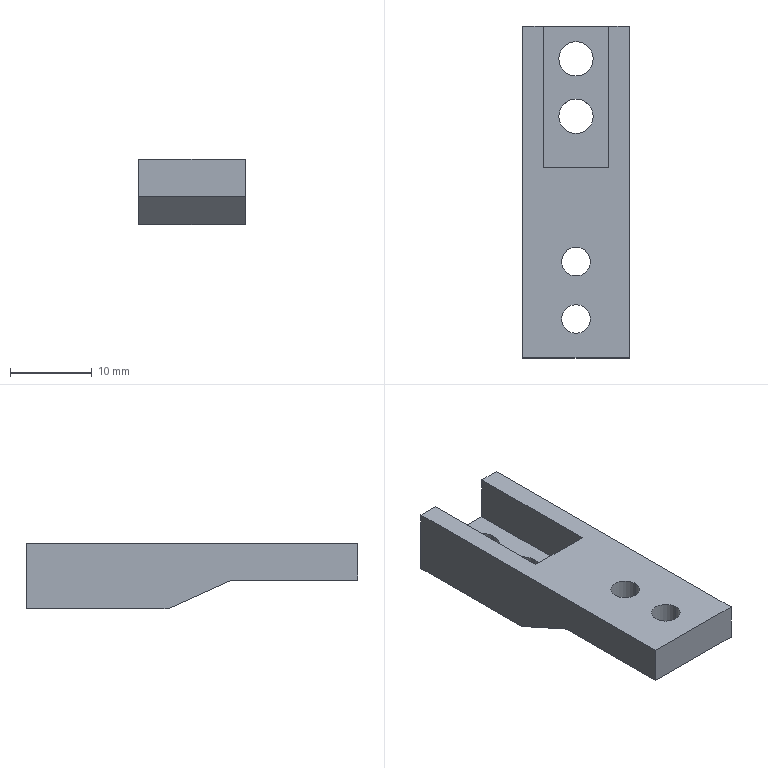Part | 1 solid | 28 faces | box 13 x 40.5 x 8 mm | volume 2407 mm3 | cylinder 12 | plane 12 | cone 4 | commonest cylinder face diameters 3.5 x4 4 x4 4.2 x4
STEP:
#1=CARTESIAN_POINT('',(1.75,-8.5,13.25));
#2=VERTEX_POINT('',#1);
#3=CARTESIAN_POINT('',(-1.75,-8.5,13.25));
#4=VERTEX_POINT('',#3);
#5=CARTESIAN_POINT('',(0.,-8.5,13.25));
#6=DIRECTION('',(0.,0.,-1.));
#7=DIRECTION('',(-1.,0.,0.));
#8=AXIS2_PLACEMENT_3D('',#5,#6,#7);
#9=CIRCLE('',#8,1.75);
#10=EDGE_CURVE('',#2,#4,#9,.T.);
#11=ORIENTED_EDGE('',*,*,#10,.F.);
#12=CARTESIAN_POINT('',(2.,-8.5,13.));
#13=VERTEX_POINT('',#12);
#14=CARTESIAN_POINT('',(2.,-8.5,13.));
#15=DIRECTION('',(0.7071,0.,-0.7071));
#16=VECTOR('',#15,1000.);
#17=LINE('',#14,#16);
#18=EDGE_CURVE('',#2,#13,#17,.T.);
#19=ORIENTED_EDGE('',*,*,#18,.T.);
#20=CARTESIAN_POINT('',(-2.,-8.5,13.));
#21=VERTEX_POINT('',#20);
#22=CARTESIAN_POINT('',(0.,-8.5,13.));
#23=DIRECTION('',(0.,0.,-1.));
#24=DIRECTION('',(-1.,0.,0.));
#25=AXIS2_PLACEMENT_3D('',#22,#23,#24);
#26=CIRCLE('',#25,2.);
#27=EDGE_CURVE('',#13,#21,#26,.T.);
#28=ORIENTED_EDGE('',*,*,#27,.T.);
#29=CARTESIAN_POINT('',(-2.,-8.5,13.));
#30=DIRECTION('',(-0.7071,0.,-0.7071));
#31=VECTOR('',#30,1000.);
#32=LINE('',#29,#31);
#33=EDGE_CURVE('',#4,#21,#32,.T.);
#34=ORIENTED_EDGE('',*,*,#33,.F.);
#35=EDGE_LOOP('',(#11,#19,#28,#34));
#36=FACE_OUTER_BOUND('',#35,.T.);
#37=CARTESIAN_POINT('',(0.,-8.5,13.));
#38=DIRECTION('',(0.,0.,-1.));
#39=DIRECTION('',(-1.,0.,0.));
#40=AXIS2_PLACEMENT_3D('',#37,#38,#39);
#41=CONICAL_SURFACE('',#40,2.,0.7854);
#42=ADVANCED_FACE('',(#36),#41,.F.);
#43=CARTESIAN_POINT('',(1.75,-15.5,13.25));
#44=VERTEX_POINT('',#43);
#45=CARTESIAN_POINT('',(-1.75,-15.5,13.25));
#46=VERTEX_POINT('',#45);
#47=CARTESIAN_POINT('',(0.,-15.5,13.25));
#48=DIRECTION('',(0.,0.,-1.));
#49=DIRECTION('',(-1.,0.,0.));
#50=AXIS2_PLACEMENT_3D('',#47,#48,#49);
#51=CIRCLE('',#50,1.75);
#52=EDGE_CURVE('',#44,#46,#51,.T.);
#53=ORIENTED_EDGE('',*,*,#52,.F.);
#54=CARTESIAN_POINT('',(2.,-15.5,13.));
#55=VERTEX_POINT('',#54);
#56=CARTESIAN_POINT('',(2.,-15.5,13.));
#57=DIRECTION('',(0.7071,0.,-0.7071));
#58=VECTOR('',#57,1000.);
#59=LINE('',#56,#58);
#60=EDGE_CURVE('',#44,#55,#59,.T.);
#61=ORIENTED_EDGE('',*,*,#60,.T.);
#62=CARTESIAN_POINT('',(-2.,-15.5,13.));
#63=VERTEX_POINT('',#62);
#64=CARTESIAN_POINT('',(0.,-15.5,13.));
#65=DIRECTION('',(0.,0.,-1.));
#66=DIRECTION('',(-1.,0.,0.));
#67=AXIS2_PLACEMENT_3D('',#64,#65,#66);
#68=CIRCLE('',#67,2.);
#69=EDGE_CURVE('',#55,#63,#68,.T.);
#70=ORIENTED_EDGE('',*,*,#69,.T.);
#71=CARTESIAN_POINT('',(-2.,-15.5,13.));
#72=DIRECTION('',(-0.7071,0.,-0.7071));
#73=VECTOR('',#72,1000.);
#74=LINE('',#71,#73);
#75=EDGE_CURVE('',#46,#63,#74,.T.);
#76=ORIENTED_EDGE('',*,*,#75,.F.);
#77=EDGE_LOOP('',(#53,#61,#70,#76));
#78=FACE_OUTER_BOUND('',#77,.T.);
#79=CARTESIAN_POINT('',(0.,-15.5,13.));
#80=DIRECTION('',(0.,0.,-1.));
#81=DIRECTION('',(-1.,0.,0.));
#82=AXIS2_PLACEMENT_3D('',#79,#80,#81);
#83=CONICAL_SURFACE('',#82,2.,0.7854);
#84=ADVANCED_FACE('',(#78),#83,.F.);
#85=ORIENTED_EDGE('',*,*,#69,.F.);
#86=CARTESIAN_POINT('',(2.,-15.5,11.5));
#87=VERTEX_POINT('',#86);
#88=CARTESIAN_POINT('',(2.,-15.5,13.));
#89=DIRECTION('',(0.,0.,-1.));
#90=VECTOR('',#89,1000.);
#91=LINE('',#88,#90);
#92=EDGE_CURVE('',#55,#87,#91,.T.);
#93=ORIENTED_EDGE('',*,*,#92,.T.);
#94=CARTESIAN_POINT('',(-2.,-15.5,11.5));
#95=VERTEX_POINT('',#94);
#96=CARTESIAN_POINT('',(0.,-15.5,11.5));
#97=DIRECTION('',(0.,0.,-1.));
#98=DIRECTION('',(-1.,0.,0.));
#99=AXIS2_PLACEMENT_3D('',#96,#97,#98);
#100=CIRCLE('',#99,2.);
#101=EDGE_CURVE('',#87,#95,#100,.T.);
#102=ORIENTED_EDGE('',*,*,#101,.T.);
#103=CARTESIAN_POINT('',(-2.,-15.5,13.));
#104=DIRECTION('',(0.,0.,-1.));
#105=VECTOR('',#104,1000.);
#106=LINE('',#103,#105);
#107=EDGE_CURVE('',#63,#95,#106,.T.);
#108=ORIENTED_EDGE('',*,*,#107,.F.);
#109=EDGE_LOOP('',(#85,#93,#102,#108));
#110=FACE_OUTER_BOUND('',#109,.T.);
#111=CARTESIAN_POINT('',(0.,-15.5,13.));
#112=DIRECTION('',(0.,0.,-1.));
#113=DIRECTION('',(-1.,0.,0.));
#114=AXIS2_PLACEMENT_3D('',#111,#112,#113);
#115=CYLINDRICAL_SURFACE('',#114,2.);
#116=ADVANCED_FACE('',(#110),#115,.F.);
#117=ORIENTED_EDGE('',*,*,#27,.F.);
#118=CARTESIAN_POINT('',(2.,-8.5,11.5));
#119=VERTEX_POINT('',#118);
#120=CARTESIAN_POINT('',(2.,-8.5,13.));
#121=DIRECTION('',(0.,0.,-1.));
#122=VECTOR('',#121,1000.);
#123=LINE('',#120,#122);
#124=EDGE_CURVE('',#13,#119,#123,.T.);
#125=ORIENTED_EDGE('',*,*,#124,.T.);
#126=CARTESIAN_POINT('',(-2.,-8.5,11.5));
#127=VERTEX_POINT('',#126);
#128=CARTESIAN_POINT('',(0.,-8.5,11.5));
#129=DIRECTION('',(0.,0.,-1.));
#130=DIRECTION('',(-1.,0.,0.));
#131=AXIS2_PLACEMENT_3D('',#128,#129,#130);
#132=CIRCLE('',#131,2.);
#133=EDGE_CURVE('',#119,#127,#132,.T.);
#134=ORIENTED_EDGE('',*,*,#133,.T.);
#135=CARTESIAN_POINT('',(-2.,-8.5,13.));
#136=DIRECTION('',(0.,0.,-1.));
#137=VECTOR('',#136,1000.);
#138=LINE('',#135,#137);
#139=EDGE_CURVE('',#21,#127,#138,.T.);
#140=ORIENTED_EDGE('',*,*,#139,.F.);
#141=EDGE_LOOP('',(#117,#125,#134,#140));
#142=FACE_OUTER_BOUND('',#141,.T.);
#143=CARTESIAN_POINT('',(0.,-8.5,13.));
#144=DIRECTION('',(0.,0.,-1.));
#145=DIRECTION('',(-1.,0.,0.));
#146=AXIS2_PLACEMENT_3D('',#143,#144,#145);
#147=CYLINDRICAL_SURFACE('',#146,2.);
#148=ADVANCED_FACE('',(#142),#147,.F.);
#149=CARTESIAN_POINT('',(-2.1,9.25,8.));
#150=VERTEX_POINT('',#149);
#151=CARTESIAN_POINT('',(2.1,9.25,8.));
#152=VERTEX_POINT('',#151);
#153=CARTESIAN_POINT('',(0.,9.25,8.));
#154=DIRECTION('',(0.,0.,1.));
#155=DIRECTION('',(0.,-1.,0.));
#156=AXIS2_PLACEMENT_3D('',#153,#154,#155);
#157=CIRCLE('',#156,2.1);
#158=EDGE_CURVE('',#150,#152,#157,.T.);
#159=ORIENTED_EDGE('',*,*,#158,.F.);
#160=CARTESIAN_POINT('',(-2.1,9.25,10.5));
#161=VERTEX_POINT('',#160);
#162=CARTESIAN_POINT('',(-2.1,9.25,0.5));
#163=DIRECTION('',(0.,0.,1.));
#164=VECTOR('',#163,1000.);
#165=LINE('',#162,#164);
#166=EDGE_CURVE('',#150,#161,#165,.T.);
#167=ORIENTED_EDGE('',*,*,#166,.T.);
#168=CARTESIAN_POINT('',(2.1,9.25,10.5));
#169=VERTEX_POINT('',#168);
#170=CARTESIAN_POINT('',(0.,9.25,10.5));
#171=DIRECTION('',(0.,0.,1.));
#172=DIRECTION('',(1.,0.,0.));
#173=AXIS2_PLACEMENT_3D('',#170,#171,#172);
#174=CIRCLE('',#173,2.1);
#175=EDGE_CURVE('',#161,#169,#174,.T.);
#176=ORIENTED_EDGE('',*,*,#175,.T.);
#177=CARTESIAN_POINT('',(2.1,9.25,0.5));
#178=DIRECTION('',(0.,0.,1.));
#179=VECTOR('',#178,1000.);
#180=LINE('',#177,#179);
#181=EDGE_CURVE('',#152,#169,#180,.T.);
#182=ORIENTED_EDGE('',*,*,#181,.F.);
#183=EDGE_LOOP('',(#159,#167,#176,#182));
#184=FACE_OUTER_BOUND('',#183,.T.);
#185=CARTESIAN_POINT('',(0.,9.25,0.5));
#186=DIRECTION('',(0.,0.,1.));
#187=DIRECTION('',(1.,0.,0.));
#188=AXIS2_PLACEMENT_3D('',#185,#186,#187);
#189=CYLINDRICAL_SURFACE('',#188,2.1);
#190=ADVANCED_FACE('',(#184),#189,.F.);
#191=CARTESIAN_POINT('',(-2.1,16.25,8.));
#192=VERTEX_POINT('',#191);
#193=CARTESIAN_POINT('',(2.1,16.25,8.));
#194=VERTEX_POINT('',#193);
#195=CARTESIAN_POINT('',(0.,16.25,8.));
#196=DIRECTION('',(0.,0.,1.));
#197=DIRECTION('',(0.,-1.,0.));
#198=AXIS2_PLACEMENT_3D('',#195,#196,#197);
#199=CIRCLE('',#198,2.1);
#200=EDGE_CURVE('',#192,#194,#199,.T.);
#201=ORIENTED_EDGE('',*,*,#200,.F.);
#202=CARTESIAN_POINT('',(-2.1,16.25,10.5));
#203=VERTEX_POINT('',#202);
#204=CARTESIAN_POINT('',(-2.1,16.25,0.5));
#205=DIRECTION('',(0.,0.,1.));
#206=VECTOR('',#205,1000.);
#207=LINE('',#204,#206);
#208=EDGE_CURVE('',#192,#203,#207,.T.);
#209=ORIENTED_EDGE('',*,*,#208,.T.);
#210=CARTESIAN_POINT('',(2.1,16.25,10.5));
#211=VERTEX_POINT('',#210);
#212=CARTESIAN_POINT('',(0.,16.25,10.5));
#213=DIRECTION('',(0.,0.,1.));
#214=DIRECTION('',(1.,0.,0.));
#215=AXIS2_PLACEMENT_3D('',#212,#213,#214);
#216=CIRCLE('',#215,2.1);
#217=EDGE_CURVE('',#203,#211,#216,.T.);
#218=ORIENTED_EDGE('',*,*,#217,.T.);
#219=CARTESIAN_POINT('',(2.1,16.25,0.5));
#220=DIRECTION('',(0.,0.,1.));
#221=VECTOR('',#220,1000.);
#222=LINE('',#219,#221);
#223=EDGE_CURVE('',#194,#211,#222,.T.);
#224=ORIENTED_EDGE('',*,*,#223,.F.);
#225=EDGE_LOOP('',(#201,#209,#218,#224));
#226=FACE_OUTER_BOUND('',#225,.T.);
#227=CARTESIAN_POINT('',(0.,16.25,0.5));
#228=DIRECTION('',(0.,0.,1.));
#229=DIRECTION('',(1.,0.,0.));
#230=AXIS2_PLACEMENT_3D('',#227,#228,#229);
#231=CYLINDRICAL_SURFACE('',#230,2.1);
#232=ADVANCED_FACE('',(#226),#231,.F.);
#233=CARTESIAN_POINT('',(1.75,-8.5,16.));
#234=VERTEX_POINT('',#233);
#235=CARTESIAN_POINT('',(-1.75,-8.5,16.));
#236=VERTEX_POINT('',#235);
#237=CARTESIAN_POINT('',(0.,-8.5,16.));
#238=DIRECTION('',(0.,0.,-1.));
#239=DIRECTION('',(-1.,0.,0.));
#240=AXIS2_PLACEMENT_3D('',#237,#238,#239);
#241=CIRCLE('',#240,1.75);
#242=EDGE_CURVE('',#234,#236,#241,.T.);
#243=ORIENTED_EDGE('',*,*,#242,.F.);
#244=CARTESIAN_POINT('',(1.75,-8.5,51.5));
#245=DIRECTION('',(0.,0.,-1.));
#246=VECTOR('',#245,1000.);
#247=LINE('',#244,#246);
#248=EDGE_CURVE('',#234,#2,#247,.T.);
#249=ORIENTED_EDGE('',*,*,#248,.T.);
#250=ORIENTED_EDGE('',*,*,#10,.T.);
#251=CARTESIAN_POINT('',(-1.75,-8.5,51.5));
#252=DIRECTION('',(0.,0.,-1.));
#253=VECTOR('',#252,1000.);
#254=LINE('',#251,#253);
#255=EDGE_CURVE('',#236,#4,#254,.T.);
#256=ORIENTED_EDGE('',*,*,#255,.F.);
#257=EDGE_LOOP('',(#243,#249,#250,#256));
#258=FACE_OUTER_BOUND('',#257,.T.);
#259=CARTESIAN_POINT('',(0.,-8.5,51.5));
#260=DIRECTION('',(0.,0.,-1.));
#261=DIRECTION('',(-1.,0.,0.));
#262=AXIS2_PLACEMENT_3D('',#259,#260,#261);
#263=CYLINDRICAL_SURFACE('',#262,1.75);
#264=ADVANCED_FACE('',(#258),#263,.F.);
#265=CARTESIAN_POINT('',(1.75,-15.5,16.));
#266=VERTEX_POINT('',#265);
#267=CARTESIAN_POINT('',(-1.75,-15.5,16.));
#268=VERTEX_POINT('',#267);
#269=CARTESIAN_POINT('',(0.,-15.5,16.));
#270=DIRECTION('',(0.,0.,-1.));
#271=DIRECTION('',(-1.,0.,0.));
#272=AXIS2_PLACEMENT_3D('',#269,#270,#271);
#273=CIRCLE('',#272,1.75);
#274=EDGE_CURVE('',#266,#268,#273,.T.);
#275=ORIENTED_EDGE('',*,*,#274,.F.);
#276=CARTESIAN_POINT('',(1.75,-15.5,51.5));
#277=DIRECTION('',(0.,0.,-1.));
#278=VECTOR('',#277,1000.);
#279=LINE('',#276,#278);
#280=EDGE_CURVE('',#266,#44,#279,.T.);
#281=ORIENTED_EDGE('',*,*,#280,.T.);
#282=ORIENTED_EDGE('',*,*,#52,.T.);
#283=CARTESIAN_POINT('',(-1.75,-15.5,51.5));
#284=DIRECTION('',(0.,0.,-1.));
#285=VECTOR('',#284,1000.);
#286=LINE('',#283,#285);
#287=EDGE_CURVE('',#268,#46,#286,.T.);
#288=ORIENTED_EDGE('',*,*,#287,.F.);
#289=EDGE_LOOP('',(#275,#281,#282,#288));
#290=FACE_OUTER_BOUND('',#289,.T.);
#291=CARTESIAN_POINT('',(0.,-15.5,51.5));
#292=DIRECTION('',(0.,0.,-1.));
#293=DIRECTION('',(-1.,0.,0.));
#294=AXIS2_PLACEMENT_3D('',#291,#292,#293);
#295=CYLINDRICAL_SURFACE('',#294,1.75);
#296=ADVANCED_FACE('',(#290),#295,.F.);
#297=ORIENTED_EDGE('',*,*,#280,.F.);
#298=CARTESIAN_POINT('',(0.,-15.5,16.));
#299=DIRECTION('',(0.,0.,-1.));
#300=DIRECTION('',(-1.,0.,0.));
#301=AXIS2_PLACEMENT_3D('',#298,#299,#300);
#302=CIRCLE('',#301,1.75);
#303=EDGE_CURVE('',#268,#266,#302,.T.);
#304=ORIENTED_EDGE('',*,*,#303,.F.);
#305=ORIENTED_EDGE('',*,*,#287,.T.);
#306=CARTESIAN_POINT('',(0.,-15.5,13.25));
#307=DIRECTION('',(0.,0.,-1.));
#308=DIRECTION('',(-1.,0.,0.));
#309=AXIS2_PLACEMENT_3D('',#306,#307,#308);
#310=CIRCLE('',#309,1.75);
#311=EDGE_CURVE('',#46,#44,#310,.T.);
#312=ORIENTED_EDGE('',*,*,#311,.T.);
#313=EDGE_LOOP('',(#297,#304,#305,#312));
#314=FACE_OUTER_BOUND('',#313,.T.);
#315=CARTESIAN_POINT('',(0.,-15.5,51.5));
#316=DIRECTION('',(0.,0.,-1.));
#317=DIRECTION('',(-1.,0.,0.));
#318=AXIS2_PLACEMENT_3D('',#315,#316,#317);
#319=CYLINDRICAL_SURFACE('',#318,1.75);
#320=ADVANCED_FACE('',(#314),#319,.F.);
#321=ORIENTED_EDGE('',*,*,#248,.F.);
#322=CARTESIAN_POINT('',(0.,-8.5,16.));
#323=DIRECTION('',(0.,0.,-1.));
#324=DIRECTION('',(-1.,0.,0.));
#325=AXIS2_PLACEMENT_3D('',#322,#323,#324);
#326=CIRCLE('',#325,1.75);
#327=EDGE_CURVE('',#236,#234,#326,.T.);
#328=ORIENTED_EDGE('',*,*,#327,.F.);
#329=ORIENTED_EDGE('',*,*,#255,.T.);
#330=CARTESIAN_POINT('',(0.,-8.5,13.25));
#331=DIRECTION('',(0.,0.,-1.));
#332=DIRECTION('',(-1.,0.,0.));
#333=AXIS2_PLACEMENT_3D('',#330,#331,#332);
#334=CIRCLE('',#333,1.75);
#335=EDGE_CURVE('',#4,#2,#334,.T.);
#336=ORIENTED_EDGE('',*,*,#335,.T.);
#337=EDGE_LOOP('',(#321,#328,#329,#336));
#338=FACE_OUTER_BOUND('',#337,.T.);
#339=CARTESIAN_POINT('',(0.,-8.5,51.5));
#340=DIRECTION('',(0.,0.,-1.));
#341=DIRECTION('',(-1.,0.,0.));
#342=AXIS2_PLACEMENT_3D('',#339,#340,#341);
#343=CYLINDRICAL_SURFACE('',#342,1.75);
#344=ADVANCED_FACE('',(#338),#343,.F.);
#345=CARTESIAN_POINT('',(-4.,2.925,10.5));
#346=VERTEX_POINT('',#345);
#347=CARTESIAN_POINT('',(-4.,2.925,16.));
#348=VERTEX_POINT('',#347);
#349=CARTESIAN_POINT('',(-4.,2.925,12.992));
#350=DIRECTION('',(0.,0.,1.));
#351=VECTOR('',#350,1000.);
#352=LINE('',#349,#351);
#353=EDGE_CURVE('',#346,#348,#352,.T.);
#354=ORIENTED_EDGE('',*,*,#353,.F.);
#355=CARTESIAN_POINT('',(-4.,20.25,10.5));
#356=VERTEX_POINT('',#355);
#357=CARTESIAN_POINT('',(-4.,-48.75,10.5));
#358=DIRECTION('',(0.,1.,0.));
#359=VECTOR('',#358,1000.);
#360=LINE('',#357,#359);
#361=EDGE_CURVE('',#346,#356,#360,.T.);
#362=ORIENTED_EDGE('',*,*,#361,.T.);
#363=CARTESIAN_POINT('',(-4.,20.25,16.));
#364=VERTEX_POINT('',#363);
#365=CARTESIAN_POINT('',(-4.,20.25,7.));
#366=DIRECTION('',(0.,0.,1.));
#367=VECTOR('',#366,1000.);
#368=LINE('',#365,#367);
#369=EDGE_CURVE('',#356,#364,#368,.T.);
#370=ORIENTED_EDGE('',*,*,#369,.T.);
#371=CARTESIAN_POINT('',(-4.,0.,16.));
#372=DIRECTION('',(0.,1.,0.));
#373=VECTOR('',#372,1000.);
#374=LINE('',#371,#373);
#375=EDGE_CURVE('',#348,#364,#374,.T.);
#376=ORIENTED_EDGE('',*,*,#375,.F.);
#377=EDGE_LOOP('',(#354,#362,#370,#376));
#378=FACE_OUTER_BOUND('',#377,.T.);
#379=CARTESIAN_POINT('',(-4.,-48.75,7.));
#380=DIRECTION('',(-1.,0.,0.));
#381=DIRECTION('',(0.,0.,1.));
#382=AXIS2_PLACEMENT_3D('',#379,#380,#381);
#383=PLANE('',#382);
#384=ADVANCED_FACE('',(#378),#383,.F.);
#385=CARTESIAN_POINT('',(4.,2.925,10.5));
#386=VERTEX_POINT('',#385);
#387=CARTESIAN_POINT('',(4.,20.25,10.5));
#388=VERTEX_POINT('',#387);
#389=CARTESIAN_POINT('',(4.,20.25,10.5));
#390=DIRECTION('',(0.,1.,0.));
#391=VECTOR('',#390,1000.);
#392=LINE('',#389,#391);
#393=EDGE_CURVE('',#386,#388,#392,.T.);
#394=ORIENTED_EDGE('',*,*,#393,.F.);
#395=CARTESIAN_POINT('',(4.,2.925,16.));
#396=VERTEX_POINT('',#395);
#397=CARTESIAN_POINT('',(4.,2.925,12.992));
#398=DIRECTION('',(0.,0.,-1.));
#399=VECTOR('',#398,1000.);
#400=LINE('',#397,#399);
#401=EDGE_CURVE('',#396,#386,#400,.T.);
#402=ORIENTED_EDGE('',*,*,#401,.F.);
#403=CARTESIAN_POINT('',(4.,20.25,16.));
#404=VERTEX_POINT('',#403);
#405=CARTESIAN_POINT('',(4.,0.,16.));
#406=DIRECTION('',(0.,-1.,0.));
#407=VECTOR('',#406,1000.);
#408=LINE('',#405,#407);
#409=EDGE_CURVE('',#404,#396,#408,.T.);
#410=ORIENTED_EDGE('',*,*,#409,.F.);
#411=CARTESIAN_POINT('',(4.,20.25,7.));
#412=DIRECTION('',(0.,0.,-1.));
#413=VECTOR('',#412,1000.);
#414=LINE('',#411,#413);
#415=EDGE_CURVE('',#404,#388,#414,.T.);
#416=ORIENTED_EDGE('',*,*,#415,.T.);
#417=EDGE_LOOP('',(#394,#402,#410,#416));
#418=FACE_OUTER_BOUND('',#417,.T.);
#419=CARTESIAN_POINT('',(4.,-48.75,7.));
#420=DIRECTION('',(1.,0.,0.));
#421=DIRECTION('',(0.,0.,-1.));
#422=AXIS2_PLACEMENT_3D('',#419,#420,#421);
#423=PLANE('',#422);
#424=ADVANCED_FACE('',(#418),#423,.F.);
#425=CARTESIAN_POINT('',(0.,9.25,10.5));
#426=DIRECTION('',(0.,0.,1.));
#427=DIRECTION('',(1.,0.,0.));
#428=AXIS2_PLACEMENT_3D('',#425,#426,#427);
#429=CIRCLE('',#428,2.1);
#430=EDGE_CURVE('',#169,#161,#429,.T.);
#431=ORIENTED_EDGE('',*,*,#430,.F.);
#432=ORIENTED_EDGE('',*,*,#175,.F.);
#433=EDGE_LOOP('',(#431,#432));
#434=FACE_BOUND('',#433,.T.);
#435=CARTESIAN_POINT('',(0.,16.25,10.5));
#436=DIRECTION('',(0.,0.,1.));
#437=DIRECTION('',(1.,0.,0.));
#438=AXIS2_PLACEMENT_3D('',#435,#436,#437);
#439=CIRCLE('',#438,2.1);
#440=EDGE_CURVE('',#211,#203,#439,.T.);
#441=ORIENTED_EDGE('',*,*,#440,.F.);
#442=ORIENTED_EDGE('',*,*,#217,.F.);
#443=EDGE_LOOP('',(#441,#442));
#444=FACE_BOUND('',#443,.T.);
#445=ORIENTED_EDGE('',*,*,#361,.F.);
#446=CARTESIAN_POINT('',(-4.,2.925,10.5));
#447=DIRECTION('',(-1.,0.,0.));
#448=VECTOR('',#447,1000.);
#449=LINE('',#446,#448);
#450=EDGE_CURVE('',#386,#346,#449,.T.);
#451=ORIENTED_EDGE('',*,*,#450,.F.);
#452=ORIENTED_EDGE('',*,*,#393,.T.);
#453=CARTESIAN_POINT('',(27.028,20.25,10.5));
#454=DIRECTION('',(-1.,0.,0.));
#455=VECTOR('',#454,1000.);
#456=LINE('',#453,#455);
#457=EDGE_CURVE('',#388,#356,#456,.T.);
#458=ORIENTED_EDGE('',*,*,#457,.T.);
#459=EDGE_LOOP('',(#445,#451,#452,#458));
#460=FACE_OUTER_BOUND('',#459,.T.);
#461=CARTESIAN_POINT('',(27.028,20.25,10.5));
#462=DIRECTION('',(0.,0.,1.));
#463=DIRECTION('',(1.,0.,0.));
#464=AXIS2_PLACEMENT_3D('',#461,#462,#463);
#465=PLANE('',#464);
#466=ADVANCED_FACE('',(#434,#444,#460),#465,.T.);
#467=CARTESIAN_POINT('',(6.5,-20.25,16.));
#468=VERTEX_POINT('',#467);
#469=CARTESIAN_POINT('',(6.5,-20.25,11.5));
#470=VERTEX_POINT('',#469);
#471=CARTESIAN_POINT('',(6.5,-20.25,16.));
#472=DIRECTION('',(0.,0.,-1.));
#473=VECTOR('',#472,1000.);
#474=LINE('',#471,#473);
#475=EDGE_CURVE('',#468,#470,#474,.T.);
#476=ORIENTED_EDGE('',*,*,#475,.T.);
#477=CARTESIAN_POINT('',(6.5,-4.869,11.5));
#478=VERTEX_POINT('',#477);
#479=CARTESIAN_POINT('',(6.5,-4.869,11.5));
#480=DIRECTION('',(0.,1.,0.));
#481=VECTOR('',#480,1000.);
#482=LINE('',#479,#481);
#483=EDGE_CURVE('',#470,#478,#482,.T.);
#484=ORIENTED_EDGE('',*,*,#483,.T.);
#485=CARTESIAN_POINT('',(6.5,2.925,8.));
#486=VERTEX_POINT('',#485);
#487=CARTESIAN_POINT('',(6.5,2.925,8.));
#488=DIRECTION('',(0.,0.9122,-0.4096));
#489=VECTOR('',#488,1000.);
#490=LINE('',#487,#489);
#491=EDGE_CURVE('',#478,#486,#490,.T.);
#492=ORIENTED_EDGE('',*,*,#491,.T.);
#493=CARTESIAN_POINT('',(6.5,20.25,8.));
#494=VERTEX_POINT('',#493);
#495=CARTESIAN_POINT('',(6.5,-20.25,8.));
#496=DIRECTION('',(0.,1.,0.));
#497=VECTOR('',#496,1000.);
#498=LINE('',#495,#497);
#499=EDGE_CURVE('',#486,#494,#498,.T.);
#500=ORIENTED_EDGE('',*,*,#499,.T.);
#501=CARTESIAN_POINT('',(6.5,20.25,16.));
#502=VERTEX_POINT('',#501);
#503=CARTESIAN_POINT('',(6.5,20.25,16.));
#504=DIRECTION('',(0.,0.,-1.));
#505=VECTOR('',#504,1000.);
#506=LINE('',#503,#505);
#507=EDGE_CURVE('',#502,#494,#506,.T.);
#508=ORIENTED_EDGE('',*,*,#507,.F.);
#509=CARTESIAN_POINT('',(6.5,-20.25,16.));
#510=DIRECTION('',(0.,1.,0.));
#511=VECTOR('',#510,1000.);
#512=LINE('',#509,#511);
#513=EDGE_CURVE('',#468,#502,#512,.T.);
#514=ORIENTED_EDGE('',*,*,#513,.F.);
#515=EDGE_LOOP('',(#476,#484,#492,#500,#508,#514));
#516=FACE_OUTER_BOUND('',#515,.T.);
#517=CARTESIAN_POINT('',(6.5,-20.25,16.));
#518=DIRECTION('',(-1.,0.,0.));
#519=DIRECTION('',(0.,0.,1.));
#520=AXIS2_PLACEMENT_3D('',#517,#518,#519);
#521=PLANE('',#520);
#522=ADVANCED_FACE('',(#516),#521,.F.);
#523=ORIENTED_EDGE('',*,*,#415,.F.);
#524=CARTESIAN_POINT('',(-6.5,20.25,16.));
#525=DIRECTION('',(-1.,0.,0.));
#526=VECTOR('',#525,1000.);
#527=LINE('',#524,#526);
#528=EDGE_CURVE('',#502,#404,#527,.T.);
#529=ORIENTED_EDGE('',*,*,#528,.F.);
#530=ORIENTED_EDGE('',*,*,#507,.T.);
#531=CARTESIAN_POINT('',(-6.5,20.25,8.));
#532=VERTEX_POINT('',#531);
#533=CARTESIAN_POINT('',(19.5,20.25,8.));
#534=DIRECTION('',(-1.,0.,0.));
#535=VECTOR('',#534,1000.);
#536=LINE('',#533,#535);
#537=EDGE_CURVE('',#494,#532,#536,.T.);
#538=ORIENTED_EDGE('',*,*,#537,.T.);
#539=CARTESIAN_POINT('',(-6.5,20.25,16.));
#540=VERTEX_POINT('',#539);
#541=CARTESIAN_POINT('',(-6.5,20.25,16.));
#542=DIRECTION('',(0.,0.,-1.));
#543=VECTOR('',#542,1000.);
#544=LINE('',#541,#543);
#545=EDGE_CURVE('',#540,#532,#544,.T.);
#546=ORIENTED_EDGE('',*,*,#545,.F.);
#547=CARTESIAN_POINT('',(-6.5,20.25,16.));
#548=DIRECTION('',(-1.,0.,0.));
#549=VECTOR('',#548,1000.);
#550=LINE('',#547,#549);
#551=EDGE_CURVE('',#364,#540,#550,.T.);
#552=ORIENTED_EDGE('',*,*,#551,.F.);
#553=ORIENTED_EDGE('',*,*,#369,.F.);
#554=ORIENTED_EDGE('',*,*,#457,.F.);
#555=EDGE_LOOP('',(#523,#529,#530,#538,#546,#552,#553,#554));
#556=FACE_OUTER_BOUND('',#555,.T.);
#557=CARTESIAN_POINT('',(-6.5,20.25,16.));
#558=DIRECTION('',(0.,-1.,0.));
#559=DIRECTION('',(0.,0.,-1.));
#560=AXIS2_PLACEMENT_3D('',#557,#558,#559);
#561=PLANE('',#560);
#562=ADVANCED_FACE('',(#556),#561,.F.);
#563=ORIENTED_EDGE('',*,*,#545,.T.);
#564=CARTESIAN_POINT('',(-6.5,2.925,8.));
#565=VERTEX_POINT('',#564);
#566=CARTESIAN_POINT('',(-6.5,20.25,8.));
#567=DIRECTION('',(0.,1.,0.));
#568=VECTOR('',#567,1000.);
#569=LINE('',#566,#568);
#570=EDGE_CURVE('',#565,#532,#569,.T.);
#571=ORIENTED_EDGE('',*,*,#570,.F.);
#572=CARTESIAN_POINT('',(-6.5,-4.869,11.5));
#573=VERTEX_POINT('',#572);
#574=CARTESIAN_POINT('',(-6.5,2.925,8.));
#575=DIRECTION('',(0.,-0.9122,0.4096));
#576=VECTOR('',#575,1000.);
#577=LINE('',#574,#576);
#578=EDGE_CURVE('',#565,#573,#577,.T.);
#579=ORIENTED_EDGE('',*,*,#578,.T.);
#580=CARTESIAN_POINT('',(-6.5,-20.25,11.5));
#581=VERTEX_POINT('',#580);
#582=CARTESIAN_POINT('',(-6.5,-4.869,11.5));
#583=DIRECTION('',(0.,-1.,0.));
#584=VECTOR('',#583,1000.);
#585=LINE('',#582,#584);
#586=EDGE_CURVE('',#573,#581,#585,.T.);
#587=ORIENTED_EDGE('',*,*,#586,.T.);
#588=CARTESIAN_POINT('',(-6.5,-20.25,16.));
#589=VERTEX_POINT('',#588);
#590=CARTESIAN_POINT('',(-6.5,-20.25,16.));
#591=DIRECTION('',(0.,0.,-1.));
#592=VECTOR('',#591,1000.);
#593=LINE('',#590,#592);
#594=EDGE_CURVE('',#589,#581,#593,.T.);
#595=ORIENTED_EDGE('',*,*,#594,.F.);
#596=CARTESIAN_POINT('',(-6.5,-20.25,16.));
#597=DIRECTION('',(0.,-1.,0.));
#598=VECTOR('',#597,1000.);
#599=LINE('',#596,#598);
#600=EDGE_CURVE('',#540,#589,#599,.T.);
#601=ORIENTED_EDGE('',*,*,#600,.F.);
#602=EDGE_LOOP('',(#563,#571,#579,#587,#595,#601));
#603=FACE_OUTER_BOUND('',#602,.T.);
#604=CARTESIAN_POINT('',(-6.5,-20.25,16.));
#605=DIRECTION('',(1.,0.,0.));
#606=DIRECTION('',(0.,0.,-1.));
#607=AXIS2_PLACEMENT_3D('',#604,#605,#606);
#608=PLANE('',#607);
#609=ADVANCED_FACE('',(#603),#608,.F.);
#610=ORIENTED_EDGE('',*,*,#594,.T.);
#611=CARTESIAN_POINT('',(30.319,-20.25,11.5));
#612=DIRECTION('',(-1.,0.,0.));
#613=VECTOR('',#612,1000.);
#614=LINE('',#611,#613);
#615=EDGE_CURVE('',#470,#581,#614,.T.);
#616=ORIENTED_EDGE('',*,*,#615,.F.);
#617=ORIENTED_EDGE('',*,*,#475,.F.);
#618=CARTESIAN_POINT('',(-6.5,-20.25,16.));
#619=DIRECTION('',(1.,0.,0.));
#620=VECTOR('',#619,1000.);
#621=LINE('',#618,#620);
#622=EDGE_CURVE('',#589,#468,#621,.T.);
#623=ORIENTED_EDGE('',*,*,#622,.F.);
#624=EDGE_LOOP('',(#610,#616,#617,#623));
#625=FACE_OUTER_BOUND('',#624,.T.);
#626=CARTESIAN_POINT('',(-6.5,-20.25,16.));
#627=DIRECTION('',(0.,1.,0.));
#628=DIRECTION('',(0.,0.,1.));
#629=AXIS2_PLACEMENT_3D('',#626,#627,#628);
#630=PLANE('',#629);
#631=ADVANCED_FACE('',(#625),#630,.F.);
#632=ORIENTED_EDGE('',*,*,#303,.T.);
#633=ORIENTED_EDGE('',*,*,#274,.T.);
#634=EDGE_LOOP('',(#632,#633));
#635=FACE_BOUND('',#634,.T.);
#636=ORIENTED_EDGE('',*,*,#327,.T.);
#637=ORIENTED_EDGE('',*,*,#242,.T.);
#638=EDGE_LOOP('',(#636,#637));
#639=FACE_BOUND('',#638,.T.);
#640=CARTESIAN_POINT('',(0.,2.925,16.));
#641=DIRECTION('',(1.,0.,0.));
#642=VECTOR('',#641,1000.);
#643=LINE('',#640,#642);
#644=EDGE_CURVE('',#348,#396,#643,.T.);
#645=ORIENTED_EDGE('',*,*,#644,.F.);
#646=ORIENTED_EDGE('',*,*,#375,.T.);
#647=ORIENTED_EDGE('',*,*,#551,.T.);
#648=ORIENTED_EDGE('',*,*,#600,.T.);
#649=ORIENTED_EDGE('',*,*,#622,.T.);
#650=ORIENTED_EDGE('',*,*,#513,.T.);
#651=ORIENTED_EDGE('',*,*,#528,.T.);
#652=ORIENTED_EDGE('',*,*,#409,.T.);
#653=EDGE_LOOP('',(#645,#646,#647,#648,#649,#650,#651,#652));
#654=FACE_OUTER_BOUND('',#653,.T.);
#655=CARTESIAN_POINT('',(0.,0.,16.));
#656=DIRECTION('',(0.,0.,-1.));
#657=DIRECTION('',(-1.,0.,0.));
#658=AXIS2_PLACEMENT_3D('',#655,#656,#657);
#659=PLANE('',#658);
#660=ADVANCED_FACE('',(#635,#639,#654),#659,.F.);
#661=CARTESIAN_POINT('',(0.,9.25,8.));
#662=DIRECTION('',(0.,0.,1.));
#663=DIRECTION('',(0.,-1.,0.));
#664=AXIS2_PLACEMENT_3D('',#661,#662,#663);
#665=CIRCLE('',#664,2.1);
#666=EDGE_CURVE('',#152,#150,#665,.T.);
#667=ORIENTED_EDGE('',*,*,#666,.T.);
#668=ORIENTED_EDGE('',*,*,#158,.T.);
#669=EDGE_LOOP('',(#667,#668));
#670=FACE_BOUND('',#669,.T.);
#671=CARTESIAN_POINT('',(0.,16.25,8.));
#672=DIRECTION('',(0.,0.,1.));
#673=DIRECTION('',(0.,-1.,0.));
#674=AXIS2_PLACEMENT_3D('',#671,#672,#673);
#675=CIRCLE('',#674,2.1);
#676=EDGE_CURVE('',#194,#192,#675,.T.);
#677=ORIENTED_EDGE('',*,*,#676,.T.);
#678=ORIENTED_EDGE('',*,*,#200,.T.);
#679=EDGE_LOOP('',(#677,#678));
#680=FACE_BOUND('',#679,.T.);
#681=ORIENTED_EDGE('',*,*,#499,.F.);
#682=CARTESIAN_POINT('',(19.5,2.925,8.));
#683=DIRECTION('',(-1.,0.,0.));
#684=VECTOR('',#683,1000.);
#685=LINE('',#682,#684);
#686=EDGE_CURVE('',#486,#565,#685,.T.);
#687=ORIENTED_EDGE('',*,*,#686,.T.);
#688=ORIENTED_EDGE('',*,*,#570,.T.);
#689=ORIENTED_EDGE('',*,*,#537,.F.);
#690=EDGE_LOOP('',(#681,#687,#688,#689));
#691=FACE_OUTER_BOUND('',#690,.T.);
#692=CARTESIAN_POINT('',(19.5,20.25,8.));
#693=DIRECTION('',(0.,0.,1.));
#694=DIRECTION('',(0.,-1.,0.));
#695=AXIS2_PLACEMENT_3D('',#692,#693,#694);
#696=PLANE('',#695);
#697=ADVANCED_FACE('',(#670,#680,#691),#696,.F.);
#698=CARTESIAN_POINT('',(0.,-15.5,11.5));
#699=DIRECTION('',(0.,0.,-1.));
#700=DIRECTION('',(-1.,0.,0.));
#701=AXIS2_PLACEMENT_3D('',#698,#699,#700);
#702=CIRCLE('',#701,2.);
#703=EDGE_CURVE('',#95,#87,#702,.T.);
#704=ORIENTED_EDGE('',*,*,#703,.F.);
#705=ORIENTED_EDGE('',*,*,#101,.F.);
#706=EDGE_LOOP('',(#704,#705));
#707=FACE_BOUND('',#706,.T.);
#708=CARTESIAN_POINT('',(0.,-8.5,11.5));
#709=DIRECTION('',(0.,0.,-1.));
#710=DIRECTION('',(-1.,0.,0.));
#711=AXIS2_PLACEMENT_3D('',#708,#709,#710);
#712=CIRCLE('',#711,2.);
#713=EDGE_CURVE('',#127,#119,#712,.T.);
#714=ORIENTED_EDGE('',*,*,#713,.F.);
#715=ORIENTED_EDGE('',*,*,#133,.F.);
#716=EDGE_LOOP('',(#714,#715));
#717=FACE_BOUND('',#716,.T.);
#718=ORIENTED_EDGE('',*,*,#483,.F.);
#719=ORIENTED_EDGE('',*,*,#615,.T.);
#720=ORIENTED_EDGE('',*,*,#586,.F.);
#721=CARTESIAN_POINT('',(30.319,-4.869,11.5));
#722=DIRECTION('',(-1.,0.,0.));
#723=VECTOR('',#722,1000.);
#724=LINE('',#721,#723);
#725=EDGE_CURVE('',#478,#573,#724,.T.);
#726=ORIENTED_EDGE('',*,*,#725,.F.);
#727=EDGE_LOOP('',(#718,#719,#720,#726));
#728=FACE_OUTER_BOUND('',#727,.T.);
#729=CARTESIAN_POINT('',(30.319,-4.869,11.5));
#730=DIRECTION('',(0.,0.,-1.));
#731=DIRECTION('',(-1.,0.,0.));
#732=AXIS2_PLACEMENT_3D('',#729,#730,#731);
#733=PLANE('',#732);
#734=ADVANCED_FACE('',(#707,#717,#728),#733,.T.);
#735=ORIENTED_EDGE('',*,*,#686,.F.);
#736=ORIENTED_EDGE('',*,*,#491,.F.);
#737=ORIENTED_EDGE('',*,*,#725,.T.);
#738=ORIENTED_EDGE('',*,*,#578,.F.);
#739=EDGE_LOOP('',(#735,#736,#737,#738));
#740=FACE_OUTER_BOUND('',#739,.T.);
#741=CARTESIAN_POINT('',(30.319,2.925,8.));
#742=DIRECTION('',(0.,-0.4096,-0.9122));
#743=DIRECTION('',(0.,0.9122,-0.4096));
#744=AXIS2_PLACEMENT_3D('',#741,#742,#743);
#745=PLANE('',#744);
#746=ADVANCED_FACE('',(#740),#745,.T.);
#747=ORIENTED_EDGE('',*,*,#644,.T.);
#748=ORIENTED_EDGE('',*,*,#401,.T.);
#749=ORIENTED_EDGE('',*,*,#450,.T.);
#750=ORIENTED_EDGE('',*,*,#353,.T.);
#751=EDGE_LOOP('',(#747,#748,#749,#750));
#752=FACE_OUTER_BOUND('',#751,.T.);
#753=CARTESIAN_POINT('',(0.,2.925,0.));
#754=DIRECTION('',(0.,1.,0.));
#755=DIRECTION('',(0.,0.,1.));
#756=AXIS2_PLACEMENT_3D('',#753,#754,#755);
#757=PLANE('',#756);
#758=ADVANCED_FACE('',(#752),#757,.T.);
#759=ORIENTED_EDGE('',*,*,#208,.F.);
#760=ORIENTED_EDGE('',*,*,#676,.F.);
#761=ORIENTED_EDGE('',*,*,#223,.T.);
#762=ORIENTED_EDGE('',*,*,#440,.T.);
#763=EDGE_LOOP('',(#759,#760,#761,#762));
#764=FACE_OUTER_BOUND('',#763,.T.);
#765=CARTESIAN_POINT('',(0.,16.25,0.5));
#766=DIRECTION('',(0.,0.,1.));
#767=DIRECTION('',(1.,0.,0.));
#768=AXIS2_PLACEMENT_3D('',#765,#766,#767);
#769=CYLINDRICAL_SURFACE('',#768,2.1);
#770=ADVANCED_FACE('',(#764),#769,.F.);
#771=ORIENTED_EDGE('',*,*,#166,.F.);
#772=ORIENTED_EDGE('',*,*,#666,.F.);
#773=ORIENTED_EDGE('',*,*,#181,.T.);
#774=ORIENTED_EDGE('',*,*,#430,.T.);
#775=EDGE_LOOP('',(#771,#772,#773,#774));
#776=FACE_OUTER_BOUND('',#775,.T.);
#777=CARTESIAN_POINT('',(0.,9.25,0.5));
#778=DIRECTION('',(0.,0.,1.));
#779=DIRECTION('',(1.,0.,0.));
#780=AXIS2_PLACEMENT_3D('',#777,#778,#779);
#781=CYLINDRICAL_SURFACE('',#780,2.1);
#782=ADVANCED_FACE('',(#776),#781,.F.);
#783=ORIENTED_EDGE('',*,*,#124,.F.);
#784=CARTESIAN_POINT('',(0.,-8.5,13.));
#785=DIRECTION('',(0.,0.,-1.));
#786=DIRECTION('',(-1.,0.,0.));
#787=AXIS2_PLACEMENT_3D('',#784,#785,#786);
#788=CIRCLE('',#787,2.);
#789=EDGE_CURVE('',#21,#13,#788,.T.);
#790=ORIENTED_EDGE('',*,*,#789,.F.);
#791=ORIENTED_EDGE('',*,*,#139,.T.);
#792=ORIENTED_EDGE('',*,*,#713,.T.);
#793=EDGE_LOOP('',(#783,#790,#791,#792));
#794=FACE_OUTER_BOUND('',#793,.T.);
#795=CARTESIAN_POINT('',(0.,-8.5,13.));
#796=DIRECTION('',(0.,0.,-1.));
#797=DIRECTION('',(-1.,0.,0.));
#798=AXIS2_PLACEMENT_3D('',#795,#796,#797);
#799=CYLINDRICAL_SURFACE('',#798,2.);
#800=ADVANCED_FACE('',(#794),#799,.F.);
#801=ORIENTED_EDGE('',*,*,#92,.F.);
#802=CARTESIAN_POINT('',(0.,-15.5,13.));
#803=DIRECTION('',(0.,0.,-1.));
#804=DIRECTION('',(-1.,0.,0.));
#805=AXIS2_PLACEMENT_3D('',#802,#803,#804);
#806=CIRCLE('',#805,2.);
#807=EDGE_CURVE('',#63,#55,#806,.T.);
#808=ORIENTED_EDGE('',*,*,#807,.F.);
#809=ORIENTED_EDGE('',*,*,#107,.T.);
#810=ORIENTED_EDGE('',*,*,#703,.T.);
#811=EDGE_LOOP('',(#801,#808,#809,#810));
#812=FACE_OUTER_BOUND('',#811,.T.);
#813=CARTESIAN_POINT('',(0.,-15.5,13.));
#814=DIRECTION('',(0.,0.,-1.));
#815=DIRECTION('',(-1.,0.,0.));
#816=AXIS2_PLACEMENT_3D('',#813,#814,#815);
#817=CYLINDRICAL_SURFACE('',#816,2.);
#818=ADVANCED_FACE('',(#812),#817,.F.);
#819=ORIENTED_EDGE('',*,*,#60,.F.);
#820=ORIENTED_EDGE('',*,*,#311,.F.);
#821=ORIENTED_EDGE('',*,*,#75,.T.);
#822=ORIENTED_EDGE('',*,*,#807,.T.);
#823=EDGE_LOOP('',(#819,#820,#821,#822));
#824=FACE_OUTER_BOUND('',#823,.T.);
#825=CARTESIAN_POINT('',(0.,-15.5,13.));
#826=DIRECTION('',(0.,0.,-1.));
#827=DIRECTION('',(-1.,0.,0.));
#828=AXIS2_PLACEMENT_3D('',#825,#826,#827);
#829=CONICAL_SURFACE('',#828,2.,0.7854);
#830=ADVANCED_FACE('',(#824),#829,.F.);
#831=ORIENTED_EDGE('',*,*,#18,.F.);
#832=ORIENTED_EDGE('',*,*,#335,.F.);
#833=ORIENTED_EDGE('',*,*,#33,.T.);
#834=ORIENTED_EDGE('',*,*,#789,.T.);
#835=EDGE_LOOP('',(#831,#832,#833,#834));
#836=FACE_OUTER_BOUND('',#835,.T.);
#837=CARTESIAN_POINT('',(0.,-8.5,13.));
#838=DIRECTION('',(0.,0.,-1.));
#839=DIRECTION('',(-1.,0.,0.));
#840=AXIS2_PLACEMENT_3D('',#837,#838,#839);
#841=CONICAL_SURFACE('',#840,2.,0.7854);
#842=ADVANCED_FACE('',(#836),#841,.F.);
#843=CLOSED_SHELL('',(#42,#84,#116,#148,#190,#232,#264,#296,#320,#344,#384,#424,#466,#522,#562,#609,#631,#660,#697,#734,#746,#758,#770,#782,#800,#818,#830,#842));
#844=MANIFOLD_SOLID_BREP('',#843);
#845=CARTESIAN_POINT('',(0.,0.,0.));
#846=DIRECTION('',(0.,0.,1.));
#847=DIRECTION('',(1.,0.,0.));
#848=AXIS2_PLACEMENT_3D('',#845,#846,#847);
#849=(LENGTH_UNIT()NAMED_UNIT(*)SI_UNIT(.MILLI.,.METRE.));
#850=UNCERTAINTY_MEASURE_WITH_UNIT(LENGTH_MEASURE(0.00001),#849,'','');
#851=(NAMED_UNIT(*)PLANE_ANGLE_UNIT()SI_UNIT($,.RADIAN.));
#852=(NAMED_UNIT(*)SI_UNIT($,.STERADIAN.)SOLID_ANGLE_UNIT());
#853=(GEOMETRIC_REPRESENTATION_CONTEXT(3)GLOBAL_UNCERTAINTY_ASSIGNED_CONTEXT((#850))GLOBAL_UNIT_ASSIGNED_CONTEXT((#849,#851,#852))REPRESENTATION_CONTEXT('',''));
#854=ADVANCED_BREP_SHAPE_REPRESENTATION('',(#844,#848),#853);